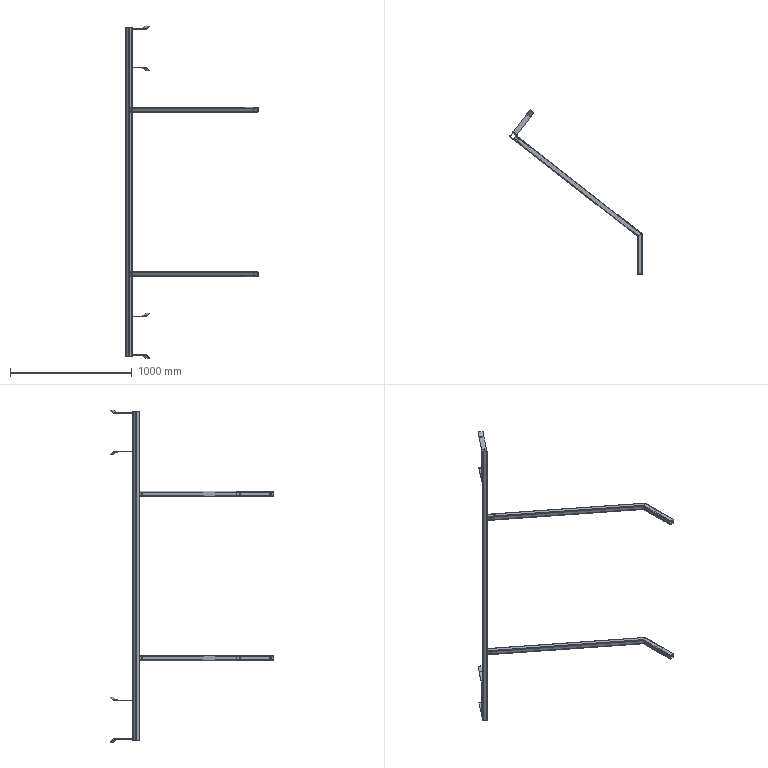Part | SolidWorks | features 3DProfileFeature 2, FlatPattern 2, ICE 2, MirrorSolid 2, MoveCopyBody 2, Stock 2, MirrorPattern 1, SheetMetal 1, WeldMemberFeat 1, WeldmentFeature 1 | 9 solids | 234 faces | box 1086 x 1346 x 2725 mm | volume 2854762 mm3 | plane 130 | cylinder 104 | commonest cylinder face diameters 12 x44 6 x28 14 x16 10 x8 20 x8